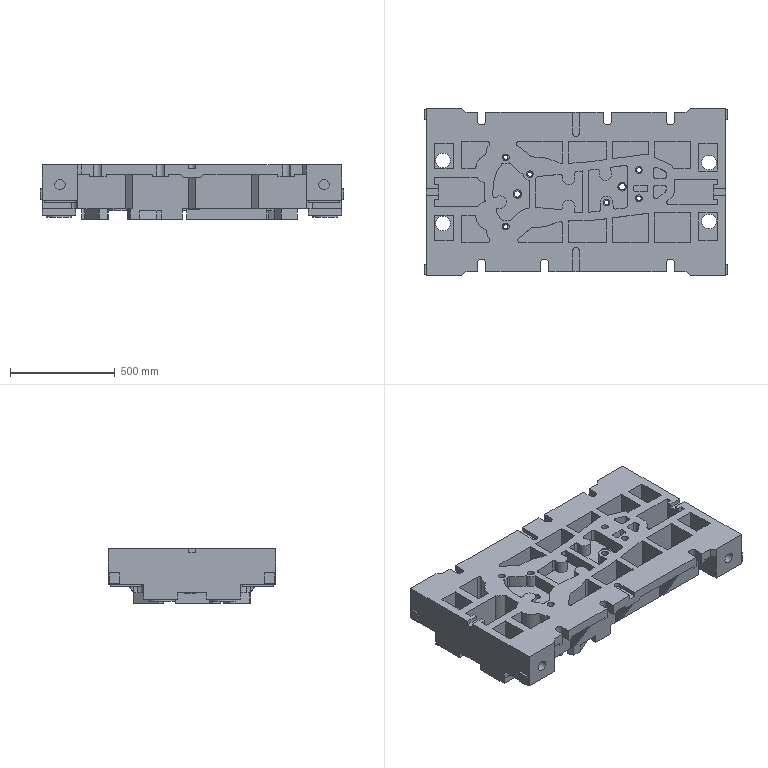Part | NX | features solid 2 | 1 solid | 631 faces | box 1450 x 800 x 260 mm | volume 132746241 mm3 | plane 446 | cylinder 152 | spline 31 | cone 2 | commonest cylinder face diameters 60 x35 20 x33 40 x22 80 x12 30 x9 32 x8